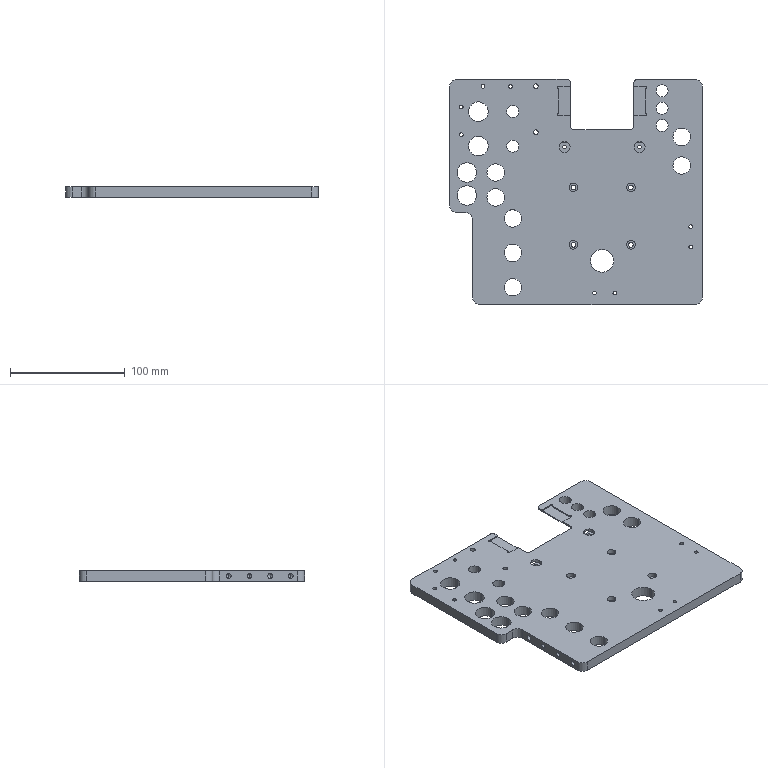NC program | NX | posted with a generic post | part box 220 x 196 x 9 mm
Lines 6261 to 7489 of 7489:
(HOLE_MILLING , TOOL : D6)
N12484 T12 M6
N12486 G54
N12488 G17 G0 G90 X-9.95 Y39.2 S9500 M3
N12490 G43 Z30. H12
N12492 Z0.5
N12494 G94 G3 X-9.075 Y38.325 R0.875 F1250.
N12496 X-8.2 Y39.2 R0.875
N12498 X-8.2 Y39.2 Z0. I-1.75 J0.
N12500 X-8.2 Y39.2 Z-0.5 I-1.75 J0.
N12502 X-8.2 Y39.2 Z-1. I-1.75 J0.
N12504 X-8.2 Y39.2 Z-1.5 I-1.75 J0.
N12506 X-8.2 Y39.2 Z-2. I-1.75 J0.
N12508 X-8.2 Y39.2 Z-2.5 I-1.75 J0.
N12510 X-8.2 Y39.2 Z-3. I-1.75 J0.
N12512 X-9.95 Y40.95 R1.75
N12514 X-8.2 Y39.2 R-1.75
N12516 X-9.075 Y40.075 R0.875
N12518 X-9.95 Y39.2 R0.875
N12520 G0 Z30.
N12522 X-2.25 Y4.
N12524 Z0.5
N12526 G3 X-1.875 Y3.625 R0.375
N12528 X-1.5 Y4. R0.375
N12530 X-1.5 Y4. Z0. I-0.75 J0.
N12532 X-1.5 Y4. Z-0.5 I-0.75 J0.
N12534 X-1.5 Y4. Z-1. I-0.75 J0.
N12536 X-1.5 Y4. Z-1.5 I-0.75 J0.
N12538 X-1.5 Y4. Z-2. I-0.75 J0.
N12540 X-1.5 Y4. Z-2.5 I-0.75 J0.
N12542 X-1.5 Y4. Z-3. I-0.75 J0.
N12544 X-1.5 Y4. Z-3.5 I-0.75 J0.
N12546 X-1.5 Y4. Z-4. I-0.75 J0.
N12548 X-2.25 Y4.75 R0.75
N12550 X-1.5 Y4. R-0.75
N12552 X-1.875 Y4.375 R0.375
N12554 X-2.25 Y4. R0.375
N12556 G0 Z30.
N12558 Y-46.
N12560 Z0.5
N12562 G3 X-1.875 Y-46.375 R0.375
N12564 X-1.5 Y-46. R0.375
N12566 X-1.5 Y-46. Z0. I-0.75 J0.
N12568 X-1.5 Y-46. Z-0.5 I-0.75 J0.
N12570 X-1.5 Y-46. Z-1. I-0.75 J0.
N12572 X-1.5 Y-46. Z-1.5 I-0.75 J0.
N12574 X-1.5 Y-46. Z-2. I-0.75 J0.
N12576 X-1.5 Y-46. Z-2.5 I-0.75 J0.
N12578 X-1.5 Y-46. Z-3. I-0.75 J0.
N12580 X-1.5 Y-46. Z-3.5 I-0.75 J0.
N12582 X-1.5 Y-46. Z-4. I-0.75 J0.
N12584 X-2.25 Y-45.25 R0.75
N12586 X-1.5 Y-46. R-0.75
N12588 X-1.875 Y-45.625 R0.375
N12590 X-2.25 Y-46. R0.375
N12592 G0 Z30.
N12594 X47.75
N12596 Z0.5
N12598 G3 X48.125 Y-46.375 R0.375
N12600 X48.5 Y-46. R0.375
N12602 X48.5 Y-46. Z0. I-0.75 J0.
N12604 X48.5 Y-46. Z-0.5 I-0.75 J0.
N12606 X48.5 Y-46. Z-1. I-0.75 J0.
N12608 X48.5 Y-46. Z-1.5 I-0.75 J0.
N12610 X48.5 Y-46. Z-2. I-0.75 J0.
N12612 X48.5 Y-46. Z-2.5 I-0.75 J0.
N12614 X48.5 Y-46. Z-3. I-0.75 J0.
N12616 X48.5 Y-46. Z-3.5 I-0.75 J0.
N12618 X48.5 Y-46. Z-4. I-0.75 J0.
N12620 X47.75 Y-45.25 R0.75
N12622 X48.5 Y-46. R-0.75
N12624 X48.125 Y-45.625 R0.375
N12626 X47.75 Y-46. R0.375
N12628 G0 Z30.
N12630 Y4.
N12632 Z0.5
N12634 G3 X48.125 Y3.625 R0.375
N12636 X48.5 Y4. R0.375
N12638 X48.5 Y4. Z0. I-0.75 J0.
N12640 X48.5 Y4. Z-0.5 I-0.75 J0.
N12642 X48.5 Y4. Z-1. I-0.75 J0.
N12644 X48.5 Y4. Z-1.5 I-0.75 J0.
N12646 X48.5 Y4. Z-2. I-0.75 J0.
N12648 X48.5 Y4. Z-2.5 I-0.75 J0.
N12650 X48.5 Y4. Z-3. I-0.75 J0.
N12652 X48.5 Y4. Z-3.5 I-0.75 J0.
N12654 X48.5 Y4. Z-4. I-0.75 J0.
N12656 X47.75 Y4.75 R0.75
N12658 X48.5 Y4. R-0.75
N12660 X48.125 Y4.375 R0.375
N12662 X47.75 Y4. R0.375
N12664 G0 Z30.
N12666 X55.35 Y39.2
N12668 Z0.5
N12670 G3 X56.225 Y38.325 R0.875
N12672 X57.1 Y39.2 R0.875
N12674 X57.1 Y39.2 Z0. I-1.75 J0.
N12676 X57.1 Y39.2 Z-0.5 I-1.75 J0.
N12678 X57.1 Y39.2 Z-1. I-1.75 J0.
N12680 X57.1 Y39.2 Z-1.5 I-1.75 J0.
N12682 X57.1 Y39.2 Z-2. I-1.75 J0.
N12684 X57.1 Y39.2 Z-2.5 I-1.75 J0.
N12686 X57.1 Y39.2 Z-3. I-1.75 J0.
N12688 X55.35 Y40.95 R1.75
N12690 X57.1 Y39.2 R-1.75
N12692 X56.225 Y40.075 R0.875
N12694 X55.35 Y39.2 R0.875
N12696 G0 Z30.
(FLOOR_WALL , TOOL : D6)
N12698 X-0.8 Y81.856
N12700 Z-0.5
N12702 G1 X-4.5 Y79.72 F1450.
N12704 G3 X-4.8 Y79.2 R0.6
N12706 G1 Y69.4
N12708 X-12.1
N12710 Y89.
N12712 X-4.8
N12714 Y79.2
N12716 X-7.8
N12718 Y72.4
N12720 X-9.1
N12722 Y86.
N12724 X-7.8
N12726 Y79.2
N12728 G3 X-7.5 Y78.68 R0.6
N12730 G0 Z30.
N12732 X-0.8 Y81.856
N12734 Z-1.
N12736 G1 X-4.5 Y79.72
N12738 G3 X-4.8 Y79.2 R0.6
N12740 G1 Y69.4
N12742 X-12.1
N12744 Y89.
N12746 X-4.8
N12748 Y79.2
N12750 X-7.8
N12752 Y72.4
N12754 X-9.1
N12756 Y86.
N12758 X-7.8
N12760 Y79.2
N12762 G3 X-7.5 Y78.68 R0.6
N12764 G0 Z30.
N12766 X46.25 Y76.544
N12768 Z-0.5
N12770 G1 X49.95 Y78.68
N12772 G3 X50.25 Y79.2 R0.6
N12774 G1 Y89.
N12776 X57.5
N12778 Y69.4
N12780 X50.25
N12782 Y79.2
N12784 X53.25
N12786 Y86.
N12788 X54.5
N12790 Y72.4
N12792 X53.25
N12794 Y79.2
N12796 G3 X52.95 Y79.72 R0.6
N12798 G0 Z30.
N12800 X46.25 Y76.544
N12802 Z-1.
N12804 G1 X49.95 Y78.68
N12806 G3 X50.25 Y79.2 R0.6
N12808 G1 Y89.
N12810 X57.5
N12812 Y69.4
N12814 X50.25
N12816 Y79.2
N12818 X53.25
N12820 Y86.
N12822 X54.5
N12824 Y72.4
N12826 X53.25
N12828 Y79.2
N12830 G3 X52.95 Y79.72 R0.6
N12832 G0 Z30.
(ZLEVEL_PROFILE_2 , TOOL : D6)
N12834 X-0.6 Y60.446
N12836 Z-0.4
N12838 G1 X-1.5 Y59.926 F1600.
N12840 G3 X-1.8 Y59.406 R0.6
N12842 G1 Y57.843
N12844 X-1.801 Y57.4
N12846 X0.206
N12848 G3 X0.726 Y57.7 R0.6
N12850 G1 X1.246 Y58.6
N12852 G0 X-0.6 Y60.446 Z-0.8
N12854 G1 X-1.5 Y59.926
N12856 G3 X-1.8 Y59.406 R0.6
N12858 G1 Y57.843
N12860 X-1.801 Y57.4
N12862 X0.206
N12864 G3 X0.726 Y57.7 R0.6
N12866 G1 X1.246 Y58.6
N12868 G0 X-0.6 Y60.446 Z-1.2
N12870 G1 X-1.5 Y59.926
N12872 G3 X-1.8 Y59.406 R0.6
N12874 G1 Y57.843
N12876 Y57.4
N12878 X0.206
N12880 G3 X0.726 Y57.7 R0.6
N12882 G1 X1.246 Y58.6
N12884 G0 X-0.6 Y60.446 Z-1.6
N12886 G1 X-1.5 Y59.926
N12888 G3 X-1.8 Y59.406 R0.6
N12890 G1 Y57.4
N12892 X0.206
N12894 G3 X0.726 Y57.7 R0.6
N12896 G1 X1.246 Y58.6
N12898 G0 Z30.
N12900 X44.204
N12902 Z-0.4
N12904 G1 X44.724 Y57.7
N12906 G3 X45.244 Y57.4 R0.6
N12908 G1 X47.25
N12910 Y59.406
N12912 G3 X46.95 Y59.926 R0.6
N12914 G1 X46.05 Y60.446
N12916 G0 X44.204 Y58.6 Z-0.8
N12918 G1 X44.724 Y57.7
N12920 G3 X45.244 Y57.4 R0.6
N12922 G1 X47.25
N12924 Y59.406
N12926 G3 X46.95 Y59.926 R0.6
N12928 G1 X46.05 Y60.446
N12930 G0 X44.204 Y58.6 Z-1.2
N12932 G1 X44.724 Y57.7
N12934 G3 X45.244 Y57.4 R0.6
N12936 G1 X47.25
N12938 Y59.406
N12940 G3 X46.95 Y59.926 R0.6
N12942 G1 X46.05 Y60.446
N12944 G0 X44.204 Y58.6 Z-1.6
N12946 G1 X44.724 Y57.7
N12948 G3 X45.244 Y57.4 R0.6
N12950 G1 X47.25
N12952 Y59.406
N12954 G3 X46.95 Y59.926 R0.6
N12956 G1 X46.05 Y60.446
N12958 G0 Z30.
N12960 M5
(ZLEVEL_PROFILE_1 , TOOL : D2)
N12962 T17 M6
N12964 G54
N12966 G17 G0 G90 X57.147 Y67.8 S9500 M3
N12968 G43 Z30. H17
N12970 Z-0.143
N12972 G94 G1 X57.32 Y67.5 F1100.
N12974 G3 X57.494 Y67.4 R0.2
N12976 G1 X60.5
N12978 G2 X59.5 Y68.4 R1.
N12980 G1 Y69.406
N12982 G3 X59.4 Y69.58 R0.2
N12984 G1 X59.1 Y69.753
N12986 G0 X57.147 Y67.8 Z-0.286
N12988 G1 X57.32 Y67.5
N12990 G3 X57.494 Y67.4 R0.2
N12992 G1 X60.5
N12994 G2 X59.5 Y68.4 R1.
N12996 G1 Y69.406
N12998 G3 X59.4 Y69.58 R0.2
N13000 G1 X59.1 Y69.753
N13002 G0 X57.147 Y67.8 Z-0.429
N13004 G1 X57.32 Y67.5
N13006 G3 X57.494 Y67.4 R0.2
N13008 G1 X60.5
N13010 G2 X59.5 Y68.4 R1.
N13012 G1 Y69.406
N13014 G3 X59.4 Y69.58 R0.2
N13016 G1 X59.1 Y69.753
N13018 G0 X57.147 Y67.8 Z-0.571
N13020 G1 X57.32 Y67.5
N13022 G3 X57.494 Y67.4 R0.2
N13024 G1 X60.5
N13026 G2 X59.5 Y68.4 R1.
N13028 G1 Y69.406
N13030 G3 X59.4 Y69.58 R0.2
N13032 G1 X59.1 Y69.753
N13034 G0 X57.147 Y67.8 Z-0.714
N13036 G1 X57.32 Y67.5
N13038 G3 X57.494 Y67.4 R0.2
N13040 G1 X60.5
N13042 G2 X59.5 Y68.4 R1.
N13044 G1 Y69.406
N13046 G3 X59.4 Y69.58 R0.2
N13048 G1 X59.1 Y69.753
N13050 G0 X57.147 Y67.8 Z-0.857
N13052 G1 X57.32 Y67.5
N13054 G3 X57.494 Y67.4 R0.2
N13056 G1 X60.5
N13058 G2 X59.5 Y68.4 R1.
N13060 G1 Y69.406
N13062 G3 X59.4 Y69.58 R0.2
N13064 G1 X59.1 Y69.753
N13066 G0 X57.147 Y67.8 Z-1.
N13068 G1 X57.32 Y67.5
N13070 G3 X57.494 Y67.4 R0.2
N13072 G1 X60.5
N13074 G2 X59.5 Y68.4 R1.
N13076 G1 Y69.406
N13078 G3 X59.4 Y69.58 R0.2
N13080 G1 X59.1 Y69.753
N13082 G0 Z30.
N13084 Y88.647
N13086 Z-0.143
N13088 G1 X59.4 Y88.82
N13090 G3 X59.5 Y88.994 R0.2
N13092 G1 Y90.
N13094 G2 X60.447 Y90.999 R1.
N13096 G1 X60.163 Y91.
N13098 X57.494
N13100 G3 X57.32 Y90.9 R0.2
N13102 G1 X57.147 Y90.6
N13104 G0 X59.1 Y88.647 Z-0.286
N13106 G1 X59.4 Y88.82
N13108 G3 X59.5 Y88.994 R0.2
N13110 G1 Y90.
N13112 G2 X60.447 Y90.999 R1.
N13114 G1 X60.163 Y91.
N13116 X57.494
N13118 G3 X57.32 Y90.9 R0.2
N13120 G1 X57.147 Y90.6
N13122 G0 X59.1 Y88.647 Z-0.429
N13124 G1 X59.4 Y88.82
N13126 G3 X59.5 Y88.994 R0.2
N13128 G1 Y90.
N13130 G2 X60.447 Y90.999 R1.
N13132 G1 X60.163 Y91.
N13134 X57.494
N13136 G3 X57.32 Y90.9 R0.2
N13138 G1 X57.147 Y90.6
N13140 G0 X59.1 Y88.647 Z-0.571
N13142 G1 X59.4 Y88.82
N13144 G3 X59.5 Y88.994 R0.2
N13146 G1 Y90.
N13148 G2 X60.447 Y90.999 R1.
N13150 G1 X60.163 Y91.
N13152 X57.494
N13154 G3 X57.32 Y90.9 R0.2
N13156 G1 X57.147 Y90.6
N13158 G0 X59.1 Y88.647 Z-0.714
N13160 G1 X59.4 Y88.82
N13162 G3 X59.5 Y88.994 R0.2
N13164 G1 Y90.
N13166 G2 X60.447 Y90.999 R1.
N13168 G1 X60.163 Y91.
N13170 X57.494
N13172 G3 X57.32 Y90.9 R0.2
N13174 G1 X57.147 Y90.6
N13176 G0 X59.1 Y88.647 Z-0.857
N13178 G1 X59.4 Y88.82
N13180 G3 X59.5 Y88.994 R0.2
N13182 G1 Y90.
N13184 G2 X60.468 Y90.999 R1.
N13186 G1 X60.163 Y91.
N13188 X57.494
N13190 G3 X57.32 Y90.9 R0.2
N13192 G1 X57.147 Y90.6
N13194 G0 X59.1 Y88.647 Z-1.
N13196 G1 X59.4 Y88.82
N13198 G3 X59.5 Y88.994 R0.2
N13200 G1 Y90.
N13202 G2 X60.449 Y90.999 R1.
N13204 G1 X60.163 Y91.
N13206 X57.494
N13208 G3 X57.32 Y90.9 R0.2
N13210 G1 X57.147 Y90.6
N13212 G0 Z30.
N13214 X-11.747
N13216 Z-0.143
N13218 G1 X-11.92 Y90.9
N13220 G3 X-12.094 Y91. R0.2
N13222 G1 X-14.752
N13224 X-15.046 Y90.999
N13226 G2 X-14.1 Y90. R1.
N13228 G1 Y88.994
N13230 G3 X-14. Y88.82 R0.2
N13232 G1 X-13.7 Y88.647
N13234 G0 X-11.747 Y90.6 Z-0.286
N13236 G1 X-11.92 Y90.9
N13238 G3 X-12.094 Y91. R0.2
N13240 G1 X-14.752
N13242 X-15.046 Y90.999
N13244 G2 X-14.1 Y90. R1.
N13246 G1 Y88.994
N13248 G3 X-14. Y88.82 R0.2
N13250 G1 X-13.7 Y88.647
N13252 G0 X-11.747 Y90.6 Z-0.429
N13254 G1 X-11.92 Y90.9
N13256 G3 X-12.094 Y91. R0.2
N13258 G1 X-14.752
N13260 X-15.046 Y90.999
N13262 G2 X-14.1 Y90. R1.
N13264 G1 Y88.994
N13266 G3 X-14. Y88.82 R0.2
N13268 G1 X-13.7 Y88.647
N13270 G0 X-11.747 Y90.6 Z-0.571
N13272 G1 X-11.92 Y90.9
N13274 G3 X-12.094 Y91. R0.2
N13276 G1 X-14.752
N13278 X-15.046 Y90.999
N13280 G2 X-14.1 Y90. R1.
N13282 G1 Y88.994
N13284 G3 X-14. Y88.82 R0.2
N13286 G1 X-13.7 Y88.647
N13288 G0 X-11.747 Y90.6 Z-0.714
N13290 G1 X-11.92 Y90.9
N13292 G3 X-12.094 Y91. R0.2
N13294 G1 X-14.752
N13296 X-15.046 Y90.999
N13298 G2 X-14.1 Y90. R1.
N13300 G1 Y88.994
N13302 G3 X-14. Y88.82 R0.2
N13304 G1 X-13.7 Y88.647
N13306 G0 X-11.747 Y90.6 Z-0.857
N13308 G1 X-11.92 Y90.9
N13310 G3 X-12.094 Y91. R0.2
N13312 G1 X-14.752
N13314 X-15.086
N13316 G2 X-14.1 Y90. R1.
N13318 G1 Y88.994
N13320 G3 X-14. Y88.82 R0.2
N13322 G1 X-13.7 Y88.647
N13324 G0 X-11.747 Y90.6 Z-1.
N13326 G1 X-11.92 Y90.9
N13328 G3 X-12.094 Y91. R0.2
N13330 G1 X-14.752
N13332 X-15.058 Y90.999
N13334 G2 X-14.1 Y90. R1.
N13336 G1 Y88.994
N13338 G3 X-14. Y88.82 R0.2
N13340 G1 X-13.7 Y88.647
N13342 G0 Z30.
N13344 Y69.753
N13346 Z-0.143
N13348 G1 X-14. Y69.58
N13350 G3 X-14.1 Y69.406 R0.2
N13352 G1 Y68.4
N13354 G2 X-15.1 Y67.4 R1.
N13356 G1 X-12.094
N13358 G3 X-11.92 Y67.5 R0.2
N13360 G1 X-11.747 Y67.8
N13362 G0 X-13.7 Y69.753 Z-0.286
N13364 G1 X-14. Y69.58
N13366 G3 X-14.1 Y69.406 R0.2
N13368 G1 Y68.4
N13370 G2 X-15.1 Y67.4 R1.
N13372 G1 X-12.094
N13374 G3 X-11.92 Y67.5 R0.2
N13376 G1 X-11.747 Y67.8
N13378 G0 X-13.7 Y69.753 Z-0.429
N13380 G1 X-14. Y69.58
N13382 G3 X-14.1 Y69.406 R0.2
N13384 G1 Y68.4
N13386 G2 X-15.1 Y67.4 R1.
N13388 G1 X-12.094
N13390 G3 X-11.92 Y67.5 R0.2
N13392 G1 X-11.747 Y67.8
N13394 G0 X-13.7 Y69.753 Z-0.571
N13396 G1 X-14. Y69.58
N13398 G3 X-14.1 Y69.406 R0.2
N13400 G1 Y68.4
N13402 G2 X-15.1 Y67.4 R1.
N13404 G1 X-12.094
N13406 G3 X-11.92 Y67.5 R0.2
N13408 G1 X-11.747 Y67.8
N13410 G0 X-13.7 Y69.753 Z-0.714
N13412 G1 X-14. Y69.58
N13414 G3 X-14.1 Y69.406 R0.2
N13416 G1 Y68.4
N13418 G2 X-15.1 Y67.4 R1.
N13420 G1 X-12.094
N13422 G3 X-11.92 Y67.5 R0.2
N13424 G1 X-11.747 Y67.8
N13426 G0 X-13.7 Y69.753 Z-0.857
N13428 G1 X-14. Y69.58
N13430 G3 X-14.1 Y69.406 R0.2
N13432 G1 Y68.4
N13434 G2 X-15.1 Y67.4 R1.
N13436 G1 X-12.094
N13438 G3 X-11.92 Y67.5 R0.2
N13440 G1 X-11.747 Y67.8
N13442 G0 X-13.7 Y69.753 Z-1.
N13444 G1 X-14. Y69.58
N13446 G3 X-14.1 Y69.406 R0.2
N13448 G1 Y68.4
N13450 G2 X-15.1 Y67.4 R1.
N13452 G1 X-12.094
N13454 G3 X-11.92 Y67.5 R0.2
N13456 G1 X-11.747 Y67.8
N13458 G0 Z30.
N13460 M5
(ZLEVEL_PROFILE_COPY_1_COPY_COPY_1_COPY , TOOL : D10JING)
N13462 T14 M6
N13464 G54
N13466 G17 G0 G90 X-70.555 Y17.229 S9500 M3
N13468 G43 Z30. H14
N13470 Z-3.5
N13472 G94 G1 Z-4.5 F1000.
N13474 X-72.1 Y17.866
N13476 G3 X-72.6 Y17. R1.
N13478 G1 Y16.98 F1200.
N13480 G3 X-69.98 Y14.4 R2.6
N13482 X-72.6 Y17. R-2.6
N13484 X-72.1 Y16.134 R1.
N13486 G1 X-70.555 Y16.771
N13488 Z-3.5
N13490 G0 Z30.
N13492 Y17.229
N13494 Z-8.
N13496 G1 Z-9. F1000.
N13498 X-72.1 Y17.866
N13500 G3 X-72.6 Y17. R1.
N13502 G1 Y16.98 F1200.
N13504 G3 X-69.98 Y14.4 R2.6
N13506 X-72.6 Y17. R-2.6
N13508 X-72.1 Y16.134 R1.
N13510 G1 X-70.555 Y16.771
N13512 Z-8.
N13514 G0 Z53.
N13516 X-96.441 Y17.416
N13518 Z-3.5
N13520 G1 Z-4.5 F1000.
N13522 X-98. Y17.866
N13524 G3 X-98.5 Y17. R1.
N13526 G1 Y16.98 F1200.
N13528 G3 X-94.98 Y13.5 R3.5
N13530 X-98.5 Y17. R-3.5
N13532 X-98. Y16.134 R1.
N13534 G1 X-96.441 Y16.584
N13536 Z-3.5
N13538 G0 Z30.
N13540 Y17.416
N13542 Z-8.
N13544 G1 Z-9. F1000.
N13546 X-98. Y17.866
N13548 G3 X-98.5 Y17. R1.
N13550 G1 Y16.98 F1200.
N13552 G3 X-94.98 Y13.5 R3.5
N13554 X-98.5 Y17. R-3.5
N13556 X-98. Y16.134 R1.
N13558 G1 X-96.441 Y16.584
N13560 Z-8.
N13562 G0 Z53.
N13564 Y-2.584
N13566 Z-3.5
N13568 G1 Z-4.5 F1000.
N13570 X-98. Y-2.134
N13572 G3 X-98.5 Y-3. R1.
N13574 G1 Y-3.02 F1200.
N13576 G3 X-94.98 Y-6.5 R3.5
N13578 X-98.5 Y-3. R-3.5
N13580 X-98. Y-3.866 R1.
N13582 G1 X-96.441 Y-3.416
N13584 Z-3.5
N13586 G0 Z30.
N13588 Y-2.584
N13590 Z-8.
N13592 G1 Z-9. F1000.
N13594 X-98. Y-2.134
N13596 G3 X-98.5 Y-3. R1.
N13598 G1 Y-3.02 F1200.
N13600 G3 X-94.98 Y-6.5 R3.5
N13602 X-98.5 Y-3. R-3.5
N13604 X-98. Y-3.866 R1.
N13606 G1 X-96.441 Y-3.416
N13608 Z-8.
N13610 G0 Z53.
N13612 X-70.555 Y-4.441
N13614 Z-3.5
N13616 G1 Z-4.5 F1000.
N13618 X-72.1 Y-3.804
N13620 G3 X-72.6 Y-4.67 R1.
N13622 X-70. Y-7.27 R2.6 F1200.
N13624 X-72.6 Y-4.67 R-2.6
N13626 X-72.1 Y-5.536 R1.
N13628 G1 X-70.555 Y-4.898
N13630 Z-3.5
N13632 G0 Z30.
N13634 Y-4.441
N13636 Z-8.
N13638 G1 Z-9. F1000.
N13640 X-72.1 Y-3.804
N13642 G3 X-72.6 Y-4.67 R1.
N13644 X-70. Y-7.27 R2.6 F1200.
N13646 X-72.6 Y-4.67 R-2.6
N13648 X-72.1 Y-5.536 R1.
N13650 G1 X-70.555 Y-4.898
N13652 Z-8.
N13654 G0 Z53.
N13656 X-86.441 Y40.416
N13658 Z-3.5
N13660 G1 Z-4.5 F1000.
N13662 X-88. Y40.866
N13664 G3 X-88.5 Y40. R1.
N13666 X-85. Y36.5 R3.5 F1200.
N13668 X-88.5 Y40. R-3.5
N13670 X-88. Y39.134 R1.
N13672 G1 X-86.441 Y39.584
N13674 Z-3.5
N13676 G0 Z30.
N13678 Y40.416
N13680 Z-8.
N13682 G1 Z-9. F1000.
N13684 X-88. Y40.866
N13686 G3 X-88.5 Y40. R1.
N13688 X-85. Y36.5 R3.5 F1200.
N13690 X-88.5 Y40. R-3.5
N13692 X-88. Y39.134 R1.
N13694 G1 X-86.441 Y39.584
N13696 Z-8.
N13698 G0 Z53.
N13700 X-55.555 Y-22.771
N13702 Z-3.5
N13704 G1 Z-4.5 F1000.
N13706 X-57.1 Y-22.134
N13708 G3 X-57.6 Y-23. R1.
N13710 G1 Y-23.02 F1200.
N13712 G3 X-54.98 Y-25.6 R2.6
N13714 X-57.6 Y-23. R-2.6
N13716 X-57.1 Y-23.866 R1.
N13718 G1 X-55.555 Y-23.229
N13720 Z-3.5
N13722 G0 Z30.
N13724 Y-22.771
N13726 Z-8.
N13728 G1 Z-9. F1000.
N13730 X-57.1 Y-22.134
N13732 G3 X-57.6 Y-23. R1.
N13734 G1 Y-23.02 F1200.
N13736 G3 X-54.98 Y-25.6 R2.6
N13738 X-57.6 Y-23. R-2.6
N13740 X-57.1 Y-23.866 R1.
N13742 G1 X-55.555 Y-23.229
N13744 Z-8.
N13746 G0 Z53.
N13748 X92.555 Y47.771
N13750 Z-3.5
N13752 G1 Z-4.5 F1000.
N13754 X94.1 Y47.134
N13756 G3 X94.6 Y48. R1.
N13758 X92. Y50.6 R2.6 F1200.
N13760 X94.6 Y48. R-2.6
N13762 X94.1 Y48.866 R1.
N13764 G1 X92.555 Y48.229
N13766 Z-3.5
N13768 G0 Z30.
N13770 Y47.771
N13772 Z-8.
N13774 G1 Z-9. F1000.
N13776 X94.1 Y47.134
N13778 G3 X94.6 Y48. R1.
N13780 X92. Y50.6 R2.6 F1200.
N13782 X94.6 Y48. R-2.6
N13784 X94.1 Y48.866 R1.
N13786 G1 X92.555 Y48.229
N13788 Z-8.
N13790 G0 Z53.
N13792 X-55.229 Y-53.555
N13794 Z-3.5
N13796 G1 Z-4.5 F1000.
N13798 X-55.866 Y-55.1
N13800 G3 X-55. Y-55.6 R1.
N13802 X-52.4 Y-53. R2.6 F1200.
N13804 X-55. Y-55.6 R-2.6
N13806 X-54.134 Y-55.1 R1.
N13808 G1 X-54.771 Y-53.555
N13810 Z-3.5
N13812 G0 Z30.
N13814 X-55.229
N13816 Z-8.
N13818 G1 Z-9. F1000.
N13820 X-55.866 Y-55.1
N13822 G3 X-55. Y-55.6 R1.
N13824 X-52.4 Y-53. R2.6 F1200.
N13826 X-55. Y-55.6 R-2.6
N13828 X-54.134 Y-55.1 R1.
N13830 G1 X-54.771 Y-53.555
N13832 Z-8.
N13834 G0 Z53.
N13836 X-86.441 Y70.416
N13838 Z-3.5
N13840 G1 Z-4.5 F1000.
N13842 X-88. Y70.866
N13844 G3 X-88.5 Y70. R1.
N13846 X-85. Y66.5 R3.5 F1200.
N13848 X-88.5 Y70. R-3.5
N13850 X-88. Y69.134 R1.
N13852 G1 X-86.441 Y69.584
N13854 Z-3.5
N13856 G0 Z30.
N13858 Y70.416
N13860 Z-8.
N13862 G1 Z-9. F1000.
N13864 X-88. Y70.866
N13866 G3 X-88.5 Y70. R1.
N13868 X-85. Y66.5 R3.5 F1200.
N13870 X-88.5 Y70. R-3.5
N13872 X-88. Y69.134 R1.
N13874 G1 X-86.441 Y69.584
N13876 Z-8.
N13878 G0 Z53.
N13880 X20.142 Y-61.501
N13882 Z-3.5
N13884 G1 Z-4.5 F1000.
N13886 X21.874 Y-64.5
N13888 G3 X22.74 Y-65. R1.
N13890 X27.74 Y-60. R5. F1200.
N13892 X22.74 Y-65. R-5.
N13894 X23.606 Y-64.5 R1.
N13896 G1 X25.338 Y-61.501
N13898 Z-3.5
N13900 G0 Z30.
N13902 X20.142
N13904 Z-8.
N13906 G1 Z-9. F1000.
N13908 X21.874 Y-64.5
N13910 G3 X22.74 Y-65. R1.
N13912 X27.74 Y-60. R5. F1200.
N13914 X22.74 Y-65. R-5.
N13916 X23.606 Y-64.5 R1.
N13918 G1 X25.338 Y-61.501
N13920 Z-8.
N13922 G0 Z53.
N13924 X92.555 Y22.771
N13926 Z-3.5
N13928 G1 Z-4.5 F1000.
N13930 X94.1 Y22.134
N13932 G3 X94.6 Y23. R1.
N13934 G1 Y23.02 F1200.
N13936 G3 X91.98 Y25.6 R2.6
N13938 X94.6 Y23. R-2.6
N13940 X94.1 Y23.866 R1.
N13942 G1 X92.555 Y23.229
N13944 Z-3.5
N13946 G0 Z30.
N13948 Y22.771
N13950 Z-8.
N13952 G1 Z-9. F1000.
N13954 X94.1 Y22.134
N13956 G3 X94.6 Y23. R1.
N13958 G1 Y23.02 F1200.
N13960 G3 X91.98 Y25.6 R2.6
N13962 X94.6 Y23. R-2.6
N13964 X94.1 Y23.866 R1.
N13966 G1 X92.555 Y23.229
N13968 Z-8.
N13970 G0 Z53.
N13972 X-55.229 Y-83.555
N13974 Z-3.5
N13976 G1 Z-4.5 F1000.
N13978 X-55.866 Y-85.1
N13980 G3 X-55. Y-85.6 R1.
N13982 X-52.4 Y-83. R2.6 F1200.
N13984 X-55. Y-85.6 R-2.6
N13986 X-54.134 Y-85.1 R1.
N13988 G1 X-54.771 Y-83.555
N13990 Z-3.5
N13992 G0 Z30.
N13994 X-55.229
N13996 Z-8.
N13998 G1 Z-9. F1000.
N14000 X-55.866 Y-85.1
N14002 G3 X-55. Y-85.6 R1.
N14004 X-52.4 Y-83. R2.6 F1200.
N14006 X-55. Y-85.6 R-2.6
N14008 X-54.134 Y-85.1 R1.
N14010 G1 X-54.771 Y-83.555
N14012 Z-8.
N14014 G0 Z30.
N14016 M5
(PLANAR_MILL_COPY_COPY_COPY_COPY_COPY_COPY_1_COPY_1 , TOOL : D6A45)
N14018 T01 M6
N14020 G54
N14022 G17 G0 G90 X-55.866 Y-89.45 S9500 M3
N14024 G43 Z30. H1
N14026 Z0.65
N14028 G94 G1 Z-0.85 F1250.
N14030 G3 X-55. Y-89.95 R1.
N14032 X-48.05 Y-83. R6.95
N14034 X-55. Y-89.95 R-6.95
N14036 X-54.134 Y-89.45 R1.
N14038 G1 Z0.65
N14040 G0 Z30.
N14042 X-55.866 Y-59.45
N14044 Z0.65
N14046 G1 Z-0.85
N14048 G3 X-55. Y-59.95 R1.
N14050 X-48.05 Y-53. R6.95
N14052 X-55. Y-59.95 R-6.95
N14054 X-54.134 Y-59.45 R1.
N14056 G1 Z0.65
N14058 G0 Z30.
N14060 X-61.45 Y-22.134
N14062 Z0.65
N14064 G1 Z-0.85
N14066 G3 X-61.95 Y-23. R1.
N14068 X-55. Y-29.95 R6.95
N14070 X-61.95 Y-23. R-6.95
N14072 X-61.45 Y-23.866 R1.
N14074 G1 Z0.65
N14076 G0 Z30.
N14078 X-76.45 Y-3.804
N14080 Z0.65
N14082 G1 Z-0.85
N14084 G3 X-76.95 Y-4.67 R1.
N14086 X-70. Y-11.62 R6.95
N14088 X-76.95 Y-4.67 R-6.95
N14090 X-76.45 Y-5.536 R1.
N14092 G1 Z0.65
N14094 G0 Z30.
N14096 X-102.35 Y-2.134
N14098 Z0.65
N14100 G1 Z-0.85
N14102 G3 X-102.85 Y-3. R1.
N14104 X-95. Y-10.85 R7.85
N14106 X-102.85 Y-3. R-7.85
N14108 X-102.35 Y-3.866 R1.
N14110 G1 Z0.65
N14112 G0 Z30.
N14114 Y17.866
N14116 Z0.65
N14118 G1 Z-0.85
N14120 G3 X-102.85 Y17. R1.
N14122 X-95. Y9.15 R7.85
N14124 X-102.85 Y17. R-7.85
N14126 X-102.35 Y16.134 R1.
N14128 G1 Z0.65
N14130 G0 Z30.
N14132 X-76.45 Y17.866
N14134 Z0.65
N14136 G1 Z-0.85
N14138 G3 X-76.95 Y17. R1.
N14140 X-70. Y10.05 R6.95
N14142 X-76.95 Y17. R-6.95
N14144 X-76.45 Y16.134 R1.
N14146 G1 Z0.65
N14148 G0 Z30.
N14150 X-92.35 Y40.866
N14152 Z0.65
N14154 G1 Z-0.85
N14156 G3 X-92.85 Y40. R1.
N14158 X-85. Y32.15 R7.85
N14160 X-92.85 Y40. R-7.85
N14162 X-92.35 Y39.134 R1.
N14164 G1 Z0.65
N14166 G0 Z30.
N14168 X-100.5 Y50.866
N14170 Z0.65
N14172 G1 Z-0.85
N14174 G3 X-101. Y50. R1.
N14176 X-100. Y49. R1.
N14178 X-101. Y50. R-1.
N14180 X-100.5 Y49.134 R1.
N14182 G1 Z0.65
N14184 G0 Z30.
N14186 Y74.866
N14188 Z0.65
N14190 G1 Z-0.85
N14192 G3 X-101. Y74. R1.
N14194 X-100. Y73. R1.
N14196 X-101. Y74. R-1.
N14198 X-100.5 Y73.134 R1.
N14200 G1 Z0.65
N14202 G0 Z30.
N14204 X-92.35 Y70.866
N14206 Z0.65
N14208 G1 Z-0.85
N14210 G3 X-92.85 Y70. R1.
N14212 X-85. Y62.15 R7.85
N14214 X-92.85 Y70. R-7.85
N14216 X-92.35 Y69.134 R1.
N14218 G1 Z0.65
N14220 G0 Z30.
N14222 X-80.134 Y92.5
N14224 Z0.65
N14226 G1 Z-0.85
N14228 G3 X-81. Y93. R1.
N14230 X-82. Y92. R1.
N14232 X-81. Y93. R-1.
N14234 X-81.866 Y92.5 R1.
N14236 G1 Z0.65
N14238 G0 Z30.
N14240 X-56.134
N14242 Z0.65
N14244 G1 Z-0.85
N14246 G3 X-57. Y93. R1.
N14248 X-58. Y92. R1.
N14250 X-57. Y93. R-1.
N14252 X-57.866 Y92.5 R1.
N14254 G1 Z0.65
N14256 G0 Z30.
N14258 X-34.134 Y92.95
N14260 Z0.65
N14262 G1 Z-0.85
N14264 G3 X-35. Y93.45 R1.
N14266 X-36.45 Y92. R1.45
N14268 X-35. Y93.45 R-1.45
N14270 X-35.866 Y92.95 R1.
N14272 G1 Z0.65
N14274 G0 Z30.
N14276 X-54.134 Y74.1
N14278 Z0.65
N14280 G1 Z-0.85
N14282 G3 X-55. Y74.6 R1.
N14284 X-59.6 Y70. R4.6
N14286 X-55. Y74.6 R-4.6
N14288 X-55.866 Y74.1 R1.
N14290 G1 Z0.65
N14292 G0 Z30.
N14294 X-59.1 Y40.866
N14296 Z0.65
N14298 G1 Z-0.85
N14300 G3 X-59.6 Y40. R1.
N14302 X-55. Y35.4 R4.6
N14304 X-59.6 Y40. R-4.6
N14306 X-59.1 Y39.134 R1.
N14308 G1 Z0.65
N14310 G0 Z30.
N14312 X-34.134 Y52.95
N14314 Z0.65
N14316 G1 Z-0.85
N14318 G3 X-35. Y53.45 R1.
N14320 X-36.45 Y52. R1.45
N14322 X-35. Y53.45 R-1.45
N14324 X-35.866 Y52.95 R1.
N14326 G1 Z0.65
N14328 G0 Z30.
N14330 X-9.084 Y42.8
N14332 Z0.65
N14334 G1 Z-0.85
N14336 G3 X-9.95 Y43.3 R1.
N14338 X-14.05 Y39.2 R4.1
N14340 X-9.95 Y43.3 R-4.1
N14342 X-10.816 Y42.8 R1.
N14344 G1 Z0.65
N14346 G0 Z30.
N14348 X-1.384 Y6.6
N14350 Z0.65
N14352 G1 Z-0.85
N14354 G3 X-2.25 Y7.1 R1.
N14356 X-5.35 Y4. R3.1
N14358 X-2.25 Y7.1 R-3.1
N14360 X-3.116 Y6.6 R1.
N14362 G1 Z0.65
N14364 G0 Z30.
N14366 X10.866 Y-99.15
N14368 Z0.65
N14370 G1 Z-0.85
N14372 G3 X10. Y-98.65 R1.
N14374 G1 X-84.
N14376 G2 X-90.65 Y-92. R6.65
N14378 G1 Y-24.
N14380 G3 X-96. Y-18.65 R5.35
N14382 G1 X-104.
N14384 G2 X-110.65 Y-12. R6.65
N14386 G1 Y92.
N14388 G2 X-104. Y98.65 R6.65
N14390 G1 X-7.8
N14392 G2 X-4.15 Y95. R3.65
N14394 G1 Y92.
N14396 G2 X-4.8 Y91.35 R0.65
N14398 G1 X-15.1
N14400 G3 X-15.45 Y91. R0.35
N14402 X-15.1 Y90.65 R0.35
N14404 G2 X-14.45 Y90. R0.65
N14406 G1 Y68.4
N14408 G2 X-15.1 Y67.75 R0.65
N14410 G3 X-15.45 Y67.4 R0.35
N14412 X-15.1 Y67.05 R0.35
N14414 G1 X-4.8
N14416 G2 X-4.15 Y66.4 R0.65
N14418 G1 Y57.4
N14420 G3 X-1.8 Y55.05 R2.35
N14422 G1 X47.25
N14424 G3 X49.6 Y57.4 R2.35
N14426 G1 Y66.4
N14428 G2 X50.25 Y67.05 R0.65
N14430 G1 X60.5
N14432 G3 X60.85 Y67.4 R0.35
N14434 X60.5 Y67.75 R0.35
N14436 G2 X59.85 Y68.4 R0.65
N14438 G1 Y90.
N14440 G2 X60.5 Y90.65 R0.65
N14442 G3 X60.85 Y91. R0.35
N14444 X60.5 Y91.35 R0.35
N14446 G1 X50.25
N14448 G2 X49.6 Y92. R0.65
N14450 G1 Y95.
N14452 G2 X53.25 Y98.65 R3.65
N14454 G1 X104.
N14456 G2 X110.65 Y92. R6.65
N14458 G1 Y-92.
N14460 G2 X104. Y-98.65 R6.65
N14462 G1 X10.
N14464 G3 X9.134 Y-99.15 R1.
N14466 G1 Z0.65
N14468 G0 Z30.
N14470 X-3.116 Y-48.6
N14472 Z0.65
N14474 G1 Z-0.85
N14476 G3 X-2.25 Y-49.1 R1.
N14478 X0.85 Y-46. R3.1
N14480 X-2.25 Y-49.1 R-3.1
N14482 X-1.384 Y-48.6 R1.
N14484 G1 Z0.65
N14486 G0 Z30.
N14488 X21.874 Y-68.85
N14490 Z0.65
N14492 G1 Z-0.85
N14494 G3 X22.74 Y-69.35 R1.
N14496 X32.09 Y-60. R9.35
N14498 X22.74 Y-69.35 R-9.35
N14500 X23.606 Y-68.85 R1.
N14502 G1 Z0.65
N14504 G0 Z30.
N14506 X15.197 Y-88.5
N14508 Z0.65
N14510 G1 Z-0.85
N14512 G3 X16.063 Y-89. R1.
N14514 X17.063 Y-88. R1.
N14516 X16.063 Y-89. R-1.
N14518 X16.929 Y-88.5 R1.
N14520 G1 Z0.65
N14522 G0 Z30.
N14524 X32.997
N14526 Z0.65
N14528 G1 Z-0.85
N14530 G3 X33.863 Y-89. R1.
N14532 X34.863 Y-88. R1.
N14534 X33.863 Y-89. R-1.
N14536 X34.729 Y-88.5 R1.
N14538 G1 Z0.65
N14540 G0 Z30.
N14542 X46.884 Y-48.6
N14544 Z0.65
N14546 G1 Z-0.85
N14548 G3 X47.75 Y-49.1 R1.
N14550 X50.85 Y-46. R3.1
N14552 X47.75 Y-49.1 R-3.1
N14554 X48.616 Y-48.6 R1.
N14556 G1 Z0.65
N14558 G0 Z30.
N14560 X50.35 Y3.134
N14562 Z0.65
N14564 G1 Z-0.85
N14566 G3 X50.85 Y4. R1.
N14568 X47.75 Y7.1 R3.1
N14570 X50.85 Y4. R-3.1
N14572 X50.35 Y4.866 R1.
N14574 G1 Z0.65
N14576 G0 Z30.
N14578 X58.95 Y38.334
N14580 Z0.65
N14582 G1 Z-0.85
N14584 G3 X59.45 Y39.2 R1.
N14586 X55.35 Y43.3 R4.1
N14588 X59.45 Y39.2 R-4.1
N14590 X58.95 Y40.066 R1.
N14592 G1 Z0.65
N14594 G0 Z30.
N14596 X79.1 Y57.134
N14598 Z0.65
N14600 G1 Z-0.85
N14602 G3 X79.6 Y58. R1.
N14604 X75. Y62.6 R4.6
N14606 X79.6 Y58. R-4.6
N14608 X79.1 Y58.866 R1.
N14610 G1 Z0.65
N14612 G0 Z30.
N14614 X75.866 Y92.1
N14616 Z0.65
N14618 G1 Z-0.85
N14620 G3 X75. Y92.6 R1.
N14622 X70.4 Y88. R4.6
N14624 X75. Y92.6 R-4.6
N14626 X74.134 Y92.1 R1.
N14628 G1 Z0.65
N14630 G0 Z30.
N14632 X75.866 Y77.1
N14634 Z0.65
N14636 G1 Z-0.85
N14638 G3 X75. Y77.6 R1.
N14640 X70.4 Y73. R4.6
N14642 X75. Y77.6 R-4.6
N14644 X74.134 Y77.1 R1.
N14646 G1 Z0.65
N14648 G0 Z30.
N14650 X98.45 Y47.134
N14652 Z0.65
N14654 G1 Z-0.85
N14656 G3 X98.95 Y48. R1.
N14658 X92. Y54.95 R6.95
N14660 X98.95 Y48. R-6.95
N14662 X98.45 Y48.866 R1.
N14664 G1 Z0.65
N14666 G0 Z30.
N14668 Y22.134
N14670 Z0.65
N14672 G1 Z-0.85
N14674 G3 X98.95 Y23. R1.
N14676 X92. Y29.95 R6.95
N14678 X98.95 Y23. R-6.95
N14680 X98.45 Y23.866 R1.
N14682 G1 Z0.65
N14684 G0 Z30.
N14686 X100.5 Y-31.066
N14688 Z0.65
N14690 G1 Z-0.85
N14692 G3 X101. Y-30.2 R1.
N14694 X100. Y-29.2 R1.
N14696 X101. Y-30.2 R-1.
N14698 X100.5 Y-29.334 R1.
N14700 G1 Z0.65
N14702 G0 Z30.
N14704 Y-48.866
N14706 Z0.65
N14708 G1 Z-0.85
N14710 G3 X101. Y-48. R1.
N14712 X100. Y-47. R1.
N14714 X101. Y-48. R-1.
N14716 X100.5 Y-47.134 R1.
N14718 G1 Z0.65
N14720 G0 Z30.
N14722 M5
(ZLEVEL_PROFILE_COPY_1_COPY_COPY_1_COPY_COPY , TOOL : D10JING)
N14724 T14 M6
N14726 G54
N14728 G17 G0 G90 X104.579 Y-103.185 S9500 M3
N14730 G43 Z30. H14
N14732 Z-7.525
N14734 G94 G1 Z-8.525 F1000.
N14736 G3 X104. Y-103. R1.
N14738 G1 X-84. F1200.
N14740 G2 X-95. Y-92. R11.
N14742 G1 Y-24.
N14744 G3 X-96. Y-23. R1.
N14746 G1 X-104.
N14748 G2 X-115. Y-12. R11.
N14750 G1 Y92.
N14752 G2 X-104. Y103. R11.
N14754 G1 X-7.8
N14756 G2 X0.2 Y95. R8.
N14758 G1 Y59.4
N14760 X45.25
N14762 Y95.
N14764 G2 X53.25 Y103. R8.
N14766 G1 X104.
N14768 G2 X115. Y92. R11.
N14770 G1 Y-92.
N14772 G2 X104. Y-103. R11.
N14774 G1 X96.839 Z-8.65
N14776 X-84.
N14778 G2 X-95. Y-92. R11.
N14780 G1 Y-24.
N14782 G3 X-96. Y-23. R1.
N14784 G1 X-104.
N14786 G2 X-115. Y-12. R11.
N14788 G1 Y92.
N14790 G2 X-104. Y103. R11.
N14792 G1 X-7.8
N14794 G2 X0.2 Y95. R8.
N14796 G1 Y59.4
N14798 X45.25
N14800 Y95.
N14802 G2 X53.25 Y103. R8.
N14804 G1 X104.
N14806 G2 X115. Y92. R11.
N14808 G1 Y-92.
N14810 G2 X104. Y-103. R11.
N14812 G1 X96.839 Z-8.775
N14814 X-84.
N14816 G2 X-95. Y-92. R11.
N14818 G1 Y-24.
N14820 G3 X-96. Y-23. R1.
N14822 G1 X-104.
N14824 G2 X-115. Y-12. R11.
N14826 G1 Y92.
N14828 G2 X-104. Y103. R11.
N14830 G1 X-7.8
N14832 G2 X0.2 Y95. R8.
N14834 G1 Y59.4
N14836 X45.25
N14838 Y95.
N14840 G2 X53.25 Y103. R8.
N14842 G1 X104.
N14844 G2 X115. Y92. R11.
N14846 G1 Y-92.
N14848 G2 X104. Y-103. R11.
N14850 G1 X96.839 Z-8.9
N14852 X-84.
N14854 G2 X-95. Y-92. R11.
N14856 G1 Y-24.
N14858 G3 X-96. Y-23. R1.
N14860 G1 X-104.
N14862 G2 X-115. Y-12. R11.
N14864 G1 Y92.
N14866 G2 X-104. Y103. R11.
N14868 G1 X-7.8
N14870 G2 X0.2 Y95. R8.
N14872 G1 Y59.4
N14874 X45.25
N14876 Y95.
N14878 G2 X53.25 Y103. R8.
N14880 G1 X104.
N14882 G2 X115. Y92. R11.
N14884 G1 Y-92.
N14886 G2 X104. Y-103. R11.
N14888 G1 X96.839
N14890 G3 X96.239 Y-103.2 R1.
N14892 G1 Z-7.9
N14894 G0 Z30.
N14896 M5
N14898 M2